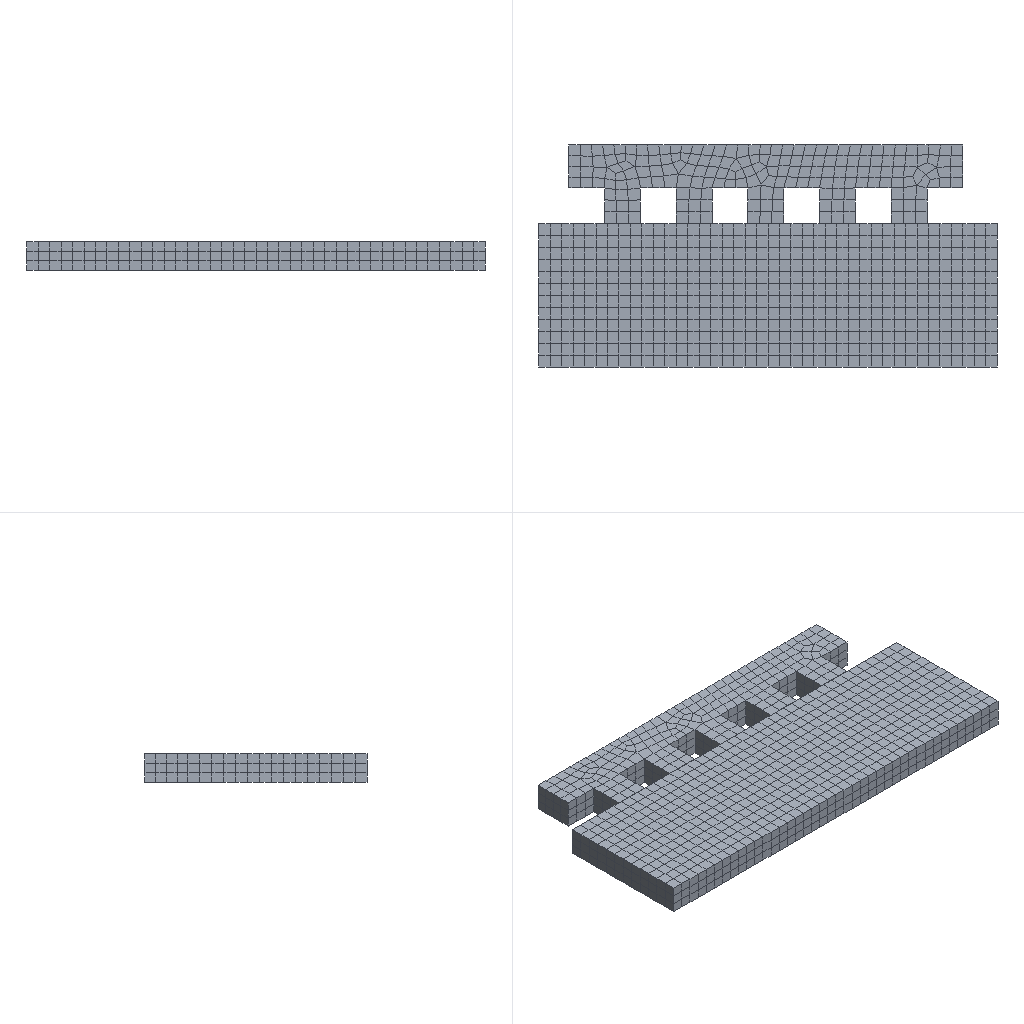Simulation study | abaqus
Set-up summary:
category,name,step,type,value,unit,region
solver,abaqus
solver,version,,,Abaqus/Explicit 2020
units,not stated in the deck,,not stated
analysis,deck,,transient,transient
load_step,Step-1,Step-1,transient
load_step,requested,,,1
mesh,nodes,,,3456
mesh,elements,,,2357
element_type,R3D4,,rigid,353
element_type,C3D8R,,solid,2004
load,load commands in deck,,count,2
bc,support commands in deck,,count,14
material,MUJU,,in results
material,WATER,,in results
check,setup vs results,,match,"per instance, exact: element labels, types and connectivity; labels of the nodes the elements use; coordinates of those nodes at SINGLE_PRECISION in 2 of 3 instance(s)"
Abaqus input file, long lists of numbers shortened:
*Heading
** Job name: Job-2 Model name: Model-1
** Generated by: Abaqus/CAE 2020
*Preprint, echo=NO, model=NO, history=NO, contact=NO
**
** PARTS
**
*Part, name=muban
*Node
      1, 0.05566, 0.02149,           0.
      2, 0.06941, 0.02149,           0.
** (966 more lines like these left out)
*Element, type=C3D8R
  1, 107, 125,  36,  35, 349, 367, 278, 277
  2, 108, 158,  78,  79, 350, 400, 320, 321
** (562 more lines like these left out)
*Nset, nset=Set-1, generate
   1,  968,    1
*Elset, elset=Set-1, generate
   1,  564,    1
** Section: muban
*Solid Section, elset=Set-1, material=muju
,
*End Part
**
*Part, name=rig
*Node
      1, 0.01125,           0., 0.001
      2, 0.01125, -0.005, 0.001
** (353 more lines like these left out)
*Element, type=R3D4
 1,   1,  17, 173,  38
 2,  17,  18, 174, 173
** (351 more lines like these left out)
*Node
    356, 0.005625,           0.,           0.
*Nset, nset=rig-RefPt_, internal
356,
*Elset, elset=rig, generate
   1,  353,    1
*End Part
**
*Part, name=water
*Node
      1, 0.07521, 0.01511, 0.001
      2, 0.07481, 0.01511, 0.001
** (2130 more lines like these left out)
*Element, type=C3D8R
   1,  165,  166,  207,  206,    1,    2,   43,   42
   2,  166,  167,  208,  207,    2,    3,   44,   43
** (1438 more lines like these left out)
*Nset, nset=Set-1, generate
    1,  2132,     1
*Elset, elset=Set-1, generate
    1,  1440,     1
** Section: wa
*Solid Section, elset=Set-1, material=water
,
*End Part
**
**
** ASSEMBLY
**
*Assembly, name=Assembly
**
*Instance, name=muban-1, part=muban
   -0.05527,    -0.02649,           0.
*End Instance
**
*Instance, name=rig-1, part=rig
     0.00125,           0.,           0.
*End Instance
**
*Instance, name=water-1, part=water
   -0.05986,    -0.02786,           0.
*End Instance
**
*Nset, nset=Set-4, instance=muban-1
   1,   2,   3,   4,   5,   6,   7,   8,   9,  10,  11,  12,  13,  14,  15,  16
  17,  18,  19,  20,  21,  22,  23,  24,  25,  26,  27,  28,  29,  30,  31,  32
** (29 more lines like these left out)
*Elset, elset=Set-4, instance=muban-1
   1,   2,   3,   4,   5,   6,   7,   8,   9,  10,  11,  12,  13,  14,  15,  16
  17,  18,  19,  20,  21,  22,  23,  24,  25,  26,  27,  28,  29,  30,  31,  32
** (22 more lines like these left out)
*Nset, nset=Set-6, instance=rig-1
 356,
*Nset, nset=Set-10, instance=water-1, generate
    1,  2132,     1
*Elset, elset=Set-10, instance=water-1, generate
    1,  1440,     1
*Nset, nset=Set-11, instance=water-1, generate
    1,  2132,     1
*Elset, elset=Set-11, instance=water-1, generate
    1,  1440,     1
*Nset, nset=Set-12, instance=water-1, generate
   1,  164,    1
*Elset, elset=Set-12, instance=water-1, generate
   1,  120,    1
*Nset, nset=Set-13, instance=water-1
    1,   41,   42,   82,   83,  123,  124,  164,  165,  205,  206,  246,  247,  287,  288,  328
  329,  369,  370,  410,  411,  451,  452,  492,  493,  533,  534,  574,  575,  615,  616,  656
** (5 more lines like these left out)
*Elset, elset=Set-13, instance=water-1
    1,   40,   41,   80,   81,  120,  121,  160,  161,  200,  201,  240,  241,  280,  281,  320
  321,  360,  361,  400,  401,  440,  441,  480,  481,  520,  521,  560,  561,  600,  601,  640
** (3 more lines like these left out)
*Nset, nset=Set-14, instance=water-1
    1,    2,    3,    4,    5,    6,    7,    8,    9,   10,   11,   12,   13,   14,   15,   16
   17,   18,   19,   20,   21,   22,   23,   24,   25,   26,   27,   28,   29,   30,   31,   32
** (65 more lines like these left out)
*Elset, elset=Set-14, instance=water-1
    1,    2,    3,    4,    5,    6,    7,    8,    9,   10,   11,   12,   13,   14,   15,   16
   17,   18,   19,   20,   21,   22,   23,   24,   25,   26,   27,   28,   29,   30,   31,   32
** (58 more lines like these left out)
*Elset, elset=_m_Surf-1_SPOS, internal, instance=rig-1
 23, 24, 25, 26, 93, 94, 95, 96, 97, 98
*Surface, type=ELEMENT, name=m_Surf-1
_m_Surf-1_SPOS, SPOS
*Elset, elset=_s_Surf-1_S5, internal, instance=muban-1
   1,   3,  11,  51, 189, 191, 199, 239, 377, 379, 387, 427
*Elset, elset=_s_Surf-1_S3, internal, instance=muban-1
  13,  14,  15,  21,  24,  26,  28,  29,  30,  33,  35,  36,  37,  38,  39,  42
  43,  44,  91, 107, 114, 124, 201, 202, 203, 209, 212, 214, 216, 217, 218, 221
** (3 more lines like these left out)
*Elset, elset=_s_Surf-1_S4, internal, instance=muban-1
  22,  23,  95, 129, 210, 211, 283, 317, 398, 399, 471, 505
*Elset, elset=_s_Surf-1_S6, internal, instance=muban-1
  46,  48,  49,  50, 105, 234, 236, 237, 238, 293, 422, 424, 425, 426, 481
*Surface, type=ELEMENT, name=s_Surf-1
_s_Surf-1_S5, S5
_s_Surf-1_S3, S3
_s_Surf-1_S4, S4
_s_Surf-1_S6, S6
*Rigid Body, ref node=rig-1.rig-RefPt_, elset=rig-1.rig
** Constraint: Constraint-1
*Tie, name=Constraint-1, adjust=yes
s_Surf-1, m_Surf-1
*End Assembly
*Amplitude, name=Amp-1
             0.,              0.,             0.1,              1.
**
** MATERIALS
**
*Material, name=muju
*Density
2000.,
*Elastic
 1e+06, 0.4
*Material, name=water
*Density
1000.,
*Eos, type=USUP
1480.,0.,0.
*Viscosity
 0.001,
**
** INTERACTION PROPERTIES
**
*Surface Interaction, name=IntProp-1
*Friction
 0.2,
*Surface Behavior, pressure-overclosure=HARD
** ----------------------------------------------------------------
**
** STEP: Step-1
**
*Step, name=Step-1, nlgeom=YES
*Dynamic, Explicit
, 0.1
*Bulk Viscosity
0.06, 1.2
** Mass Scaling: Semi-Automatic
**               Whole Model
*Fixed Mass Scaling, factor=500.
**
** BOUNDARY CONDITIONS
**
** Name: BC-1 Type: 位移/转角
*Boundary
Set-14, 3, 3
** Name: BC-2 Type: 位移/转角
*Boundary
Set-13, 1, 1
** Name: BC-3 Type: 位移/转角
*Boundary
Set-12, 1, 1
Set-12, 2, 2
Set-12, 3, 3
Set-12, 4, 4
Set-12, 5, 5
Set-12, 6, 6
** Name: BC-5 Type: 位移/转角
*Boundary, amplitude=Amp-1
Set-6, 1, 1
Set-6, 2, 2, -0.0015
Set-6, 3, 3
Set-6, 4, 4
Set-6, 5, 5
Set-6, 6, 6
**
** LOADS
**
** Name: Load-1   Type: Gravity
*Dload
Set-10, GRAV, 9.8, 0., -1., 0.
**
** INTERACTIONS
**
** Interaction: Int-1
*Contact, op=NEW
*Contact Inclusions, ALL EXTERIOR
*Contact Property Assignment
 ,  , IntProp-1
**
** OUTPUT REQUESTS
**
*Restart, write, number interval=1, time marks=NO
**
** FIELD OUTPUT: F-Output-1
**
*Output, field, number interval=50
*Node Output
A, CF, RF, RM, RT, U, V
*Element Output, directions=YES
DENSITY, DENSITYVAVG, E, EACTIVE, EVF, LE, MISES, MISESMAX, MISESONLY, PE, PEEQ, PEEQVAVG, PEVAVG, S, SSAVG, SVAVG
*Contact Output
CDISP, CSTRESS
**
** HISTORY OUTPUT: H-Output-1
**
*Output, history, variable=PRESELECT
*End Step
Results summary:
result,step,Step-1,partial,increments=1073392 time=0.08257/0.1
result,analysis,,,transient
result,last_loadstep,,,1
result,primary field,,,U
result,reaction total,,FX,0.002768,model units
result,reaction total,,FY,0.02308,model units
result,reaction total,,FZ,2.1e-05,model units